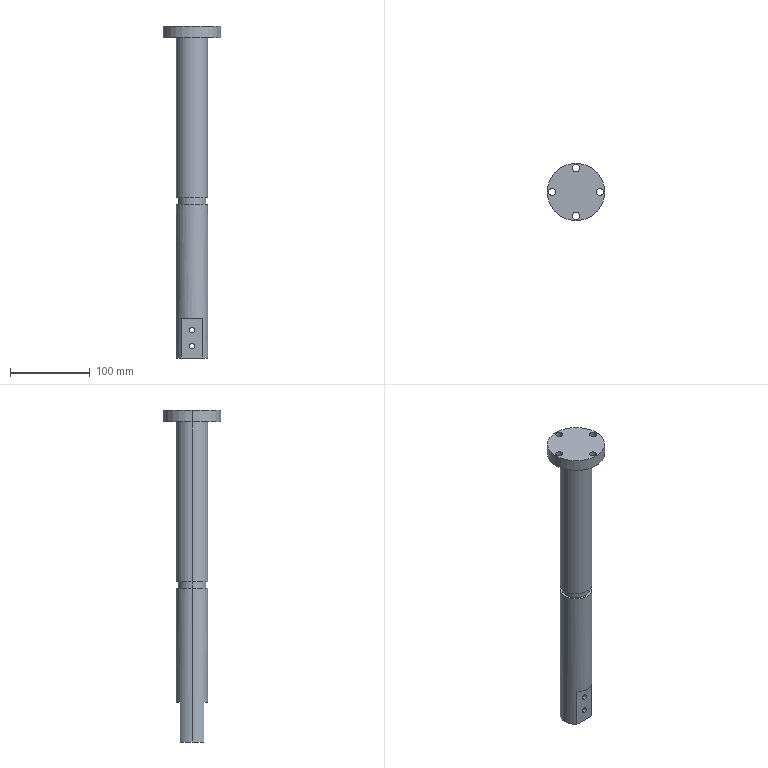Part | SolidWorks | features BaseBody 1 | 1 solid | 29 faces | box 72 x 72 x 416.14 mm | volume 547741 mm3 | cylinder 20 | plane 9 | commonest cylinder face diameters 9 x8 6.8 x4 40 x4 35 x2 72 x2
STEP:
#1=CARTESIAN_POINT('',(-20.,0.,-32.879));
#2=VERTEX_POINT('',#1);
#3=CARTESIAN_POINT('',(20.,0.,-32.879));
#4=VERTEX_POINT('',#3);
#5=CARTESIAN_POINT('',(0.,0.,-32.879));
#6=DIRECTION('',(0.,0.,-1.));
#7=DIRECTION('',(-1.,0.,0.));
#8=AXIS2_PLACEMENT_3D('',#5,#6,#7);
#9=CIRCLE('',#8,20.);
#10=EDGE_CURVE('',#2,#4,#9,.T.);
#11=ORIENTED_EDGE('',*,*,#10,.T.);
#12=CARTESIAN_POINT('',(20.,0.,-233.243));
#13=VERTEX_POINT('',#12);
#14=CARTESIAN_POINT('',(20.,0.,-32.879));
#15=DIRECTION('',(0.,0.,-1.));
#16=VECTOR('',#15,1000.);
#17=LINE('',#14,#16);
#18=EDGE_CURVE('',#4,#13,#17,.T.);
#19=ORIENTED_EDGE('',*,*,#18,.T.);
#20=CARTESIAN_POINT('',(-20.,0.,-233.243));
#21=VERTEX_POINT('',#20);
#22=CARTESIAN_POINT('',(0.,0.,-233.243));
#23=DIRECTION('',(0.,0.,1.));
#24=DIRECTION('',(-1.,0.,0.));
#25=AXIS2_PLACEMENT_3D('',#22,#23,#24);
#26=CIRCLE('',#25,20.);
#27=EDGE_CURVE('',#13,#21,#26,.T.);
#28=ORIENTED_EDGE('',*,*,#27,.T.);
#29=CARTESIAN_POINT('',(-20.,0.,-32.879));
#30=DIRECTION('',(0.,0.,-1.));
#31=VECTOR('',#30,1000.);
#32=LINE('',#29,#31);
#33=EDGE_CURVE('',#2,#21,#32,.T.);
#34=ORIENTED_EDGE('',*,*,#33,.F.);
#35=EDGE_LOOP('',(#11,#19,#28,#34));
#36=FACE_OUTER_BOUND('',#35,.T.);
#37=CARTESIAN_POINT('',(0.,0.,-32.879));
#38=DIRECTION('',(0.,0.,-1.));
#39=DIRECTION('',(-1.,0.,0.));
#40=AXIS2_PLACEMENT_3D('',#37,#38,#39);
#41=CYLINDRICAL_SURFACE('',#40,20.);
#42=ADVANCED_FACE('',(#36),#41,.T.);
#43=CARTESIAN_POINT('',(-17.5,0.,-233.243));
#44=VERTEX_POINT('',#43);
#45=CARTESIAN_POINT('',(17.5,0.,-233.243));
#46=VERTEX_POINT('',#45);
#47=CARTESIAN_POINT('',(0.,0.,-233.243));
#48=DIRECTION('',(0.,0.,-1.));
#49=DIRECTION('',(-1.,0.,0.));
#50=AXIS2_PLACEMENT_3D('',#47,#48,#49);
#51=CIRCLE('',#50,17.5);
#52=EDGE_CURVE('',#44,#46,#51,.T.);
#53=ORIENTED_EDGE('',*,*,#52,.T.);
#54=CARTESIAN_POINT('',(17.5,0.,-241.243));
#55=VERTEX_POINT('',#54);
#56=CARTESIAN_POINT('',(17.5,0.,-434.019));
#57=DIRECTION('',(0.,0.,-1.));
#58=VECTOR('',#57,1000.);
#59=LINE('',#56,#58);
#60=EDGE_CURVE('',#46,#55,#59,.T.);
#61=ORIENTED_EDGE('',*,*,#60,.T.);
#62=CARTESIAN_POINT('',(-17.5,0.,-241.243));
#63=VERTEX_POINT('',#62);
#64=CARTESIAN_POINT('',(0.,0.,-241.243));
#65=DIRECTION('',(0.,0.,1.));
#66=DIRECTION('',(-1.,0.,0.));
#67=AXIS2_PLACEMENT_3D('',#64,#65,#66);
#68=CIRCLE('',#67,17.5);
#69=EDGE_CURVE('',#55,#63,#68,.T.);
#70=ORIENTED_EDGE('',*,*,#69,.T.);
#71=CARTESIAN_POINT('',(-17.5,0.,-434.019));
#72=DIRECTION('',(0.,0.,-1.));
#73=VECTOR('',#72,1000.);
#74=LINE('',#71,#73);
#75=EDGE_CURVE('',#44,#63,#74,.T.);
#76=ORIENTED_EDGE('',*,*,#75,.F.);
#77=EDGE_LOOP('',(#53,#61,#70,#76));
#78=FACE_OUTER_BOUND('',#77,.T.);
#79=CARTESIAN_POINT('',(0.,0.,-434.019));
#80=DIRECTION('',(0.,0.,-1.));
#81=DIRECTION('',(-1.,0.,0.));
#82=AXIS2_PLACEMENT_3D('',#79,#80,#81);
#83=CYLINDRICAL_SURFACE('',#82,17.5);
#84=ADVANCED_FACE('',(#78),#83,.T.);
#85=CARTESIAN_POINT('',(-36.,0.,-17.879));
#86=VERTEX_POINT('',#85);
#87=CARTESIAN_POINT('',(36.,0.,-17.879));
#88=VERTEX_POINT('',#87);
#89=CARTESIAN_POINT('',(0.,0.,-17.879));
#90=DIRECTION('',(0.,0.,-1.));
#91=DIRECTION('',(-1.,0.,0.));
#92=AXIS2_PLACEMENT_3D('',#89,#90,#91);
#93=CIRCLE('',#92,36.);
#94=EDGE_CURVE('',#86,#88,#93,.T.);
#95=ORIENTED_EDGE('',*,*,#94,.T.);
#96=CARTESIAN_POINT('',(36.,0.,-32.879));
#97=VERTEX_POINT('',#96);
#98=CARTESIAN_POINT('',(36.,0.,-17.879));
#99=DIRECTION('',(0.,0.,-1.));
#100=VECTOR('',#99,1000.);
#101=LINE('',#98,#100);
#102=EDGE_CURVE('',#88,#97,#101,.T.);
#103=ORIENTED_EDGE('',*,*,#102,.T.);
#104=CARTESIAN_POINT('',(-36.,0.,-32.879));
#105=VERTEX_POINT('',#104);
#106=CARTESIAN_POINT('',(0.,0.,-32.879));
#107=DIRECTION('',(0.,0.,1.));
#108=DIRECTION('',(-1.,0.,0.));
#109=AXIS2_PLACEMENT_3D('',#106,#107,#108);
#110=CIRCLE('',#109,36.);
#111=EDGE_CURVE('',#97,#105,#110,.T.);
#112=ORIENTED_EDGE('',*,*,#111,.T.);
#113=CARTESIAN_POINT('',(-36.,0.,-17.879));
#114=DIRECTION('',(0.,0.,-1.));
#115=VECTOR('',#114,1000.);
#116=LINE('',#113,#115);
#117=EDGE_CURVE('',#86,#105,#116,.T.);
#118=ORIENTED_EDGE('',*,*,#117,.F.);
#119=EDGE_LOOP('',(#95,#103,#112,#118));
#120=FACE_OUTER_BOUND('',#119,.T.);
#121=CARTESIAN_POINT('',(0.,0.,-17.879));
#122=DIRECTION('',(0.,0.,-1.));
#123=DIRECTION('',(-1.,0.,0.));
#124=AXIS2_PLACEMENT_3D('',#121,#122,#123);
#125=CYLINDRICAL_SURFACE('',#124,36.);
#126=ADVANCED_FACE('',(#120),#125,.T.);
#127=CARTESIAN_POINT('',(4.5,30.,-32.879));
#128=VERTEX_POINT('',#127);
#129=CARTESIAN_POINT('',(-4.5,30.,-32.879));
#130=VERTEX_POINT('',#129);
#131=CARTESIAN_POINT('',(0.,30.,-32.879));
#132=DIRECTION('',(0.,0.,-1.));
#133=DIRECTION('',(1.,0.,0.));
#134=AXIS2_PLACEMENT_3D('',#131,#132,#133);
#135=CIRCLE('',#134,4.5);
#136=EDGE_CURVE('',#128,#130,#135,.T.);
#137=ORIENTED_EDGE('',*,*,#136,.T.);
#138=CARTESIAN_POINT('',(-4.5,30.,-17.879));
#139=VERTEX_POINT('',#138);
#140=CARTESIAN_POINT('',(-4.5,30.,-434.02));
#141=DIRECTION('',(0.,0.,1.));
#142=VECTOR('',#141,1000.);
#143=LINE('',#140,#142);
#144=EDGE_CURVE('',#130,#139,#143,.T.);
#145=ORIENTED_EDGE('',*,*,#144,.T.);
#146=CARTESIAN_POINT('',(4.5,30.,-17.879));
#147=VERTEX_POINT('',#146);
#148=CARTESIAN_POINT('',(0.,30.,-17.879));
#149=DIRECTION('',(0.,0.,-1.));
#150=DIRECTION('',(1.,0.,0.));
#151=AXIS2_PLACEMENT_3D('',#148,#149,#150);
#152=CIRCLE('',#151,4.5);
#153=EDGE_CURVE('',#147,#139,#152,.T.);
#154=ORIENTED_EDGE('',*,*,#153,.F.);
#155=CARTESIAN_POINT('',(4.5,30.,-434.02));
#156=DIRECTION('',(0.,0.,1.));
#157=VECTOR('',#156,1000.);
#158=LINE('',#155,#157);
#159=EDGE_CURVE('',#128,#147,#158,.T.);
#160=ORIENTED_EDGE('',*,*,#159,.F.);
#161=EDGE_LOOP('',(#137,#145,#154,#160));
#162=FACE_OUTER_BOUND('',#161,.T.);
#163=CARTESIAN_POINT('',(0.,30.,-434.02));
#164=DIRECTION('',(0.,0.,1.));
#165=DIRECTION('',(1.,0.,0.));
#166=AXIS2_PLACEMENT_3D('',#163,#164,#165);
#167=CYLINDRICAL_SURFACE('',#166,4.5);
#168=ADVANCED_FACE('',(#162),#167,.F.);
#169=CARTESIAN_POINT('',(-25.5,0.,-32.879));
#170=VERTEX_POINT('',#169);
#171=CARTESIAN_POINT('',(-34.5,0.,-32.879));
#172=VERTEX_POINT('',#171);
#173=CARTESIAN_POINT('',(-30.,0.,-32.879));
#174=DIRECTION('',(0.,0.,-1.));
#175=DIRECTION('',(1.,0.,0.));
#176=AXIS2_PLACEMENT_3D('',#173,#174,#175);
#177=CIRCLE('',#176,4.5);
#178=EDGE_CURVE('',#170,#172,#177,.T.);
#179=ORIENTED_EDGE('',*,*,#178,.T.);
#180=CARTESIAN_POINT('',(-34.5,0.,-17.879));
#181=VERTEX_POINT('',#180);
#182=CARTESIAN_POINT('',(-34.5,0.,-434.02));
#183=DIRECTION('',(0.,0.,1.));
#184=VECTOR('',#183,1000.);
#185=LINE('',#182,#184);
#186=EDGE_CURVE('',#172,#181,#185,.T.);
#187=ORIENTED_EDGE('',*,*,#186,.T.);
#188=CARTESIAN_POINT('',(-25.5,0.,-17.879));
#189=VERTEX_POINT('',#188);
#190=CARTESIAN_POINT('',(-30.,0.,-17.879));
#191=DIRECTION('',(0.,0.,-1.));
#192=DIRECTION('',(1.,0.,0.));
#193=AXIS2_PLACEMENT_3D('',#190,#191,#192);
#194=CIRCLE('',#193,4.5);
#195=EDGE_CURVE('',#189,#181,#194,.T.);
#196=ORIENTED_EDGE('',*,*,#195,.F.);
#197=CARTESIAN_POINT('',(-25.5,0.,-434.02));
#198=DIRECTION('',(0.,0.,1.));
#199=VECTOR('',#198,1000.);
#200=LINE('',#197,#199);
#201=EDGE_CURVE('',#170,#189,#200,.T.);
#202=ORIENTED_EDGE('',*,*,#201,.F.);
#203=EDGE_LOOP('',(#179,#187,#196,#202));
#204=FACE_OUTER_BOUND('',#203,.T.);
#205=CARTESIAN_POINT('',(-30.,0.,-434.02));
#206=DIRECTION('',(0.,0.,1.));
#207=DIRECTION('',(1.,0.,0.));
#208=AXIS2_PLACEMENT_3D('',#205,#206,#207);
#209=CYLINDRICAL_SURFACE('',#208,4.5);
#210=ADVANCED_FACE('',(#204),#209,.F.);
#211=CARTESIAN_POINT('',(4.5,-30.,-32.879));
#212=VERTEX_POINT('',#211);
#213=CARTESIAN_POINT('',(-4.5,-30.,-32.879));
#214=VERTEX_POINT('',#213);
#215=CARTESIAN_POINT('',(0.,-30.,-32.879));
#216=DIRECTION('',(0.,0.,-1.));
#217=DIRECTION('',(1.,0.,0.));
#218=AXIS2_PLACEMENT_3D('',#215,#216,#217);
#219=CIRCLE('',#218,4.5);
#220=EDGE_CURVE('',#212,#214,#219,.T.);
#221=ORIENTED_EDGE('',*,*,#220,.T.);
#222=CARTESIAN_POINT('',(-4.5,-30.,-17.879));
#223=VERTEX_POINT('',#222);
#224=CARTESIAN_POINT('',(-4.5,-30.,-434.02));
#225=DIRECTION('',(0.,0.,1.));
#226=VECTOR('',#225,1000.);
#227=LINE('',#224,#226);
#228=EDGE_CURVE('',#214,#223,#227,.T.);
#229=ORIENTED_EDGE('',*,*,#228,.T.);
#230=CARTESIAN_POINT('',(4.5,-30.,-17.879));
#231=VERTEX_POINT('',#230);
#232=CARTESIAN_POINT('',(0.,-30.,-17.879));
#233=DIRECTION('',(0.,0.,-1.));
#234=DIRECTION('',(1.,0.,0.));
#235=AXIS2_PLACEMENT_3D('',#232,#233,#234);
#236=CIRCLE('',#235,4.5);
#237=EDGE_CURVE('',#231,#223,#236,.T.);
#238=ORIENTED_EDGE('',*,*,#237,.F.);
#239=CARTESIAN_POINT('',(4.5,-30.,-434.02));
#240=DIRECTION('',(0.,0.,1.));
#241=VECTOR('',#240,1000.);
#242=LINE('',#239,#241);
#243=EDGE_CURVE('',#212,#231,#242,.T.);
#244=ORIENTED_EDGE('',*,*,#243,.F.);
#245=EDGE_LOOP('',(#221,#229,#238,#244));
#246=FACE_OUTER_BOUND('',#245,.T.);
#247=CARTESIAN_POINT('',(0.,-30.,-434.02));
#248=DIRECTION('',(0.,0.,1.));
#249=DIRECTION('',(1.,0.,0.));
#250=AXIS2_PLACEMENT_3D('',#247,#248,#249);
#251=CYLINDRICAL_SURFACE('',#250,4.5);
#252=ADVANCED_FACE('',(#246),#251,.F.);
#253=CARTESIAN_POINT('',(34.5,0.,-32.879));
#254=VERTEX_POINT('',#253);
#255=CARTESIAN_POINT('',(25.5,0.,-32.879));
#256=VERTEX_POINT('',#255);
#257=CARTESIAN_POINT('',(30.,0.,-32.879));
#258=DIRECTION('',(0.,0.,-1.));
#259=DIRECTION('',(1.,0.,0.));
#260=AXIS2_PLACEMENT_3D('',#257,#258,#259);
#261=CIRCLE('',#260,4.5);
#262=EDGE_CURVE('',#254,#256,#261,.T.);
#263=ORIENTED_EDGE('',*,*,#262,.T.);
#264=CARTESIAN_POINT('',(25.5,0.,-17.879));
#265=VERTEX_POINT('',#264);
#266=CARTESIAN_POINT('',(25.5,0.,-434.02));
#267=DIRECTION('',(0.,0.,1.));
#268=VECTOR('',#267,1000.);
#269=LINE('',#266,#268);
#270=EDGE_CURVE('',#256,#265,#269,.T.);
#271=ORIENTED_EDGE('',*,*,#270,.T.);
#272=CARTESIAN_POINT('',(34.5,0.,-17.879));
#273=VERTEX_POINT('',#272);
#274=CARTESIAN_POINT('',(30.,0.,-17.879));
#275=DIRECTION('',(0.,0.,-1.));
#276=DIRECTION('',(1.,0.,0.));
#277=AXIS2_PLACEMENT_3D('',#274,#275,#276);
#278=CIRCLE('',#277,4.5);
#279=EDGE_CURVE('',#273,#265,#278,.T.);
#280=ORIENTED_EDGE('',*,*,#279,.F.);
#281=CARTESIAN_POINT('',(34.5,0.,-434.02));
#282=DIRECTION('',(0.,0.,1.));
#283=VECTOR('',#282,1000.);
#284=LINE('',#281,#283);
#285=EDGE_CURVE('',#254,#273,#284,.T.);
#286=ORIENTED_EDGE('',*,*,#285,.F.);
#287=EDGE_LOOP('',(#263,#271,#280,#286));
#288=FACE_OUTER_BOUND('',#287,.T.);
#289=CARTESIAN_POINT('',(30.,0.,-434.02));
#290=DIRECTION('',(0.,0.,1.));
#291=DIRECTION('',(1.,0.,0.));
#292=AXIS2_PLACEMENT_3D('',#289,#290,#291);
#293=CYLINDRICAL_SURFACE('',#292,4.5);
#294=ADVANCED_FACE('',(#288),#293,.F.);
#295=CARTESIAN_POINT('',(20.,0.,-241.243));
#296=VERTEX_POINT('',#295);
#297=CARTESIAN_POINT('',(-20.,0.,-241.243));
#298=VERTEX_POINT('',#297);
#299=CARTESIAN_POINT('',(0.,0.,-241.243));
#300=DIRECTION('',(0.,0.,1.));
#301=DIRECTION('',(-1.,0.,0.));
#302=AXIS2_PLACEMENT_3D('',#299,#300,#301);
#303=CIRCLE('',#302,20.);
#304=EDGE_CURVE('',#296,#298,#303,.T.);
#305=ORIENTED_EDGE('',*,*,#304,.F.);
#306=CARTESIAN_POINT('',(20.,0.,-434.019));
#307=VERTEX_POINT('',#306);
#308=CARTESIAN_POINT('',(20.,0.,-32.879));
#309=DIRECTION('',(0.,0.,-1.));
#310=VECTOR('',#309,1000.);
#311=LINE('',#308,#310);
#312=EDGE_CURVE('',#296,#307,#311,.T.);
#313=ORIENTED_EDGE('',*,*,#312,.T.);
#314=CARTESIAN_POINT('',(13.229,15.,-434.019));
#315=VERTEX_POINT('',#314);
#316=CARTESIAN_POINT('',(0.,0.,-434.019));
#317=DIRECTION('',(0.,0.,1.));
#318=DIRECTION('',(-1.,0.,0.));
#319=AXIS2_PLACEMENT_3D('',#316,#317,#318);
#320=CIRCLE('',#319,20.);
#321=EDGE_CURVE('',#307,#315,#320,.T.);
#322=ORIENTED_EDGE('',*,*,#321,.T.);
#323=CARTESIAN_POINT('',(13.229,15.,-384.019));
#324=VERTEX_POINT('',#323);
#325=CARTESIAN_POINT('',(13.229,15.,-32.879));
#326=DIRECTION('',(0.,0.,1.));
#327=VECTOR('',#326,1000.);
#328=LINE('',#325,#327);
#329=EDGE_CURVE('',#315,#324,#328,.T.);
#330=ORIENTED_EDGE('',*,*,#329,.T.);
#331=CARTESIAN_POINT('',(-13.229,15.,-384.019));
#332=VERTEX_POINT('',#331);
#333=CARTESIAN_POINT('',(0.,0.,-384.019));
#334=DIRECTION('',(0.,0.,1.));
#335=DIRECTION('',(-1.,0.,0.));
#336=AXIS2_PLACEMENT_3D('',#333,#334,#335);
#337=CIRCLE('',#336,20.);
#338=EDGE_CURVE('',#324,#332,#337,.T.);
#339=ORIENTED_EDGE('',*,*,#338,.T.);
#340=CARTESIAN_POINT('',(-13.229,15.,-434.019));
#341=VERTEX_POINT('',#340);
#342=CARTESIAN_POINT('',(-13.229,15.,-32.879));
#343=DIRECTION('',(0.,0.,-1.));
#344=VECTOR('',#343,1000.);
#345=LINE('',#342,#344);
#346=EDGE_CURVE('',#332,#341,#345,.T.);
#347=ORIENTED_EDGE('',*,*,#346,.T.);
#348=CARTESIAN_POINT('',(-20.,0.,-434.019));
#349=VERTEX_POINT('',#348);
#350=CARTESIAN_POINT('',(0.,0.,-434.019));
#351=DIRECTION('',(0.,0.,1.));
#352=DIRECTION('',(-1.,0.,0.));
#353=AXIS2_PLACEMENT_3D('',#350,#351,#352);
#354=CIRCLE('',#353,20.);
#355=EDGE_CURVE('',#341,#349,#354,.T.);
#356=ORIENTED_EDGE('',*,*,#355,.T.);
#357=CARTESIAN_POINT('',(-20.,0.,-32.879));
#358=DIRECTION('',(0.,0.,-1.));
#359=VECTOR('',#358,1000.);
#360=LINE('',#357,#359);
#361=EDGE_CURVE('',#298,#349,#360,.T.);
#362=ORIENTED_EDGE('',*,*,#361,.F.);
#363=EDGE_LOOP('',(#305,#313,#322,#330,#339,#347,#356,#362));
#364=FACE_OUTER_BOUND('',#363,.T.);
#365=CARTESIAN_POINT('',(0.,0.,-32.879));
#366=DIRECTION('',(0.,0.,-1.));
#367=DIRECTION('',(-1.,0.,0.));
#368=AXIS2_PLACEMENT_3D('',#365,#366,#367);
#369=CYLINDRICAL_SURFACE('',#368,20.);
#370=ADVANCED_FACE('',(#364),#369,.T.);
#371=CARTESIAN_POINT('',(0.,-15.,-422.419));
#372=VERTEX_POINT('',#371);
#373=CARTESIAN_POINT('',(0.,-15.,-415.619));
#374=VERTEX_POINT('',#373);
#375=CARTESIAN_POINT('',(0.,-15.,-419.019));
#376=DIRECTION('',(0.,1.,0.));
#377=DIRECTION('',(0.,0.,1.));
#378=AXIS2_PLACEMENT_3D('',#375,#376,#377);
#379=CIRCLE('',#378,3.4);
#380=EDGE_CURVE('',#372,#374,#379,.T.);
#381=ORIENTED_EDGE('',*,*,#380,.F.);
#382=CARTESIAN_POINT('',(0.,15.,-422.419));
#383=VERTEX_POINT('',#382);
#384=CARTESIAN_POINT('',(0.,15.,-422.419));
#385=DIRECTION('',(0.,1.,0.));
#386=VECTOR('',#385,1000.);
#387=LINE('',#384,#386);
#388=EDGE_CURVE('',#372,#383,#387,.T.);
#389=ORIENTED_EDGE('',*,*,#388,.T.);
#390=CARTESIAN_POINT('',(0.,15.,-415.619));
#391=VERTEX_POINT('',#390);
#392=CARTESIAN_POINT('',(0.,15.,-419.019));
#393=DIRECTION('',(0.,1.,0.));
#394=DIRECTION('',(0.,0.,1.));
#395=AXIS2_PLACEMENT_3D('',#392,#393,#394);
#396=CIRCLE('',#395,3.4);
#397=EDGE_CURVE('',#383,#391,#396,.T.);
#398=ORIENTED_EDGE('',*,*,#397,.T.);
#399=CARTESIAN_POINT('',(0.,15.,-415.619));
#400=DIRECTION('',(0.,1.,0.));
#401=VECTOR('',#400,1000.);
#402=LINE('',#399,#401);
#403=EDGE_CURVE('',#374,#391,#402,.T.);
#404=ORIENTED_EDGE('',*,*,#403,.F.);
#405=EDGE_LOOP('',(#381,#389,#398,#404));
#406=FACE_OUTER_BOUND('',#405,.T.);
#407=CARTESIAN_POINT('',(0.,15.,-419.019));
#408=DIRECTION('',(0.,1.,0.));
#409=DIRECTION('',(0.,0.,1.));
#410=AXIS2_PLACEMENT_3D('',#407,#408,#409);
#411=CYLINDRICAL_SURFACE('',#410,3.4);
#412=ADVANCED_FACE('',(#406),#411,.F.);
#413=CARTESIAN_POINT('',(0.,-15.,-402.419));
#414=VERTEX_POINT('',#413);
#415=CARTESIAN_POINT('',(0.,-15.,-395.619));
#416=VERTEX_POINT('',#415);
#417=CARTESIAN_POINT('',(0.,-15.,-399.019));
#418=DIRECTION('',(0.,1.,0.));
#419=DIRECTION('',(0.,0.,1.));
#420=AXIS2_PLACEMENT_3D('',#417,#418,#419);
#421=CIRCLE('',#420,3.4);
#422=EDGE_CURVE('',#414,#416,#421,.T.);
#423=ORIENTED_EDGE('',*,*,#422,.F.);
#424=CARTESIAN_POINT('',(0.,15.,-402.419));
#425=VERTEX_POINT('',#424);
#426=CARTESIAN_POINT('',(0.,15.,-402.419));
#427=DIRECTION('',(0.,1.,0.));
#428=VECTOR('',#427,1000.);
#429=LINE('',#426,#428);
#430=EDGE_CURVE('',#414,#425,#429,.T.);
#431=ORIENTED_EDGE('',*,*,#430,.T.);
#432=CARTESIAN_POINT('',(0.,15.,-395.619));
#433=VERTEX_POINT('',#432);
#434=CARTESIAN_POINT('',(0.,15.,-399.019));
#435=DIRECTION('',(0.,1.,0.));
#436=DIRECTION('',(0.,0.,1.));
#437=AXIS2_PLACEMENT_3D('',#434,#435,#436);
#438=CIRCLE('',#437,3.4);
#439=EDGE_CURVE('',#425,#433,#438,.T.);
#440=ORIENTED_EDGE('',*,*,#439,.T.);
#441=CARTESIAN_POINT('',(0.,15.,-395.619));
#442=DIRECTION('',(0.,1.,0.));
#443=VECTOR('',#442,1000.);
#444=LINE('',#441,#443);
#445=EDGE_CURVE('',#416,#433,#444,.T.);
#446=ORIENTED_EDGE('',*,*,#445,.F.);
#447=EDGE_LOOP('',(#423,#431,#440,#446));
#448=FACE_OUTER_BOUND('',#447,.T.);
#449=CARTESIAN_POINT('',(0.,15.,-399.019));
#450=DIRECTION('',(0.,1.,0.));
#451=DIRECTION('',(0.,0.,1.));
#452=AXIS2_PLACEMENT_3D('',#449,#450,#451);
#453=CYLINDRICAL_SURFACE('',#452,3.4);
#454=ADVANCED_FACE('',(#448),#453,.F.);
#455=ORIENTED_EDGE('',*,*,#18,.F.);
#456=CARTESIAN_POINT('',(0.,0.,-32.879));
#457=DIRECTION('',(0.,0.,-1.));
#458=DIRECTION('',(-1.,0.,0.));
#459=AXIS2_PLACEMENT_3D('',#456,#457,#458);
#460=CIRCLE('',#459,20.);
#461=EDGE_CURVE('',#4,#2,#460,.T.);
#462=ORIENTED_EDGE('',*,*,#461,.T.);
#463=ORIENTED_EDGE('',*,*,#33,.T.);
#464=CARTESIAN_POINT('',(0.,0.,-233.243));
#465=DIRECTION('',(0.,0.,1.));
#466=DIRECTION('',(-1.,0.,0.));
#467=AXIS2_PLACEMENT_3D('',#464,#465,#466);
#468=CIRCLE('',#467,20.);
#469=EDGE_CURVE('',#21,#13,#468,.T.);
#470=ORIENTED_EDGE('',*,*,#469,.T.);
#471=EDGE_LOOP('',(#455,#462,#463,#470));
#472=FACE_OUTER_BOUND('',#471,.T.);
#473=CARTESIAN_POINT('',(0.,0.,-32.879));
#474=DIRECTION('',(0.,0.,-1.));
#475=DIRECTION('',(-1.,0.,0.));
#476=AXIS2_PLACEMENT_3D('',#473,#474,#475);
#477=CYLINDRICAL_SURFACE('',#476,20.);
#478=ADVANCED_FACE('',(#472),#477,.T.);
#479=ORIENTED_EDGE('',*,*,#469,.F.);
#480=ORIENTED_EDGE('',*,*,#27,.F.);
#481=EDGE_LOOP('',(#479,#480));
#482=FACE_OUTER_BOUND('',#481,.T.);
#483=ORIENTED_EDGE('',*,*,#52,.F.);
#484=CARTESIAN_POINT('',(0.,0.,-233.243));
#485=DIRECTION('',(0.,0.,-1.));
#486=DIRECTION('',(-1.,0.,0.));
#487=AXIS2_PLACEMENT_3D('',#484,#485,#486);
#488=CIRCLE('',#487,17.5);
#489=EDGE_CURVE('',#46,#44,#488,.T.);
#490=ORIENTED_EDGE('',*,*,#489,.F.);
#491=EDGE_LOOP('',(#483,#490));
#492=FACE_BOUND('',#491,.T.);
#493=CARTESIAN_POINT('',(0.,-20.,-233.243));
#494=DIRECTION('',(0.,0.,1.));
#495=DIRECTION('',(1.,0.,0.));
#496=AXIS2_PLACEMENT_3D('',#493,#494,#495);
#497=PLANE('',#496);
#498=ADVANCED_FACE('',(#482,#492),#497,.F.);
#499=ORIENTED_EDGE('',*,*,#10,.F.);
#500=ORIENTED_EDGE('',*,*,#461,.F.);
#501=EDGE_LOOP('',(#499,#500));
#502=FACE_BOUND('',#501,.T.);
#503=CARTESIAN_POINT('',(0.,0.,-32.879));
#504=DIRECTION('',(0.,0.,1.));
#505=DIRECTION('',(-1.,0.,0.));
#506=AXIS2_PLACEMENT_3D('',#503,#504,#505);
#507=CIRCLE('',#506,36.);
#508=EDGE_CURVE('',#105,#97,#507,.T.);
#509=ORIENTED_EDGE('',*,*,#508,.F.);
#510=ORIENTED_EDGE('',*,*,#111,.F.);
#511=EDGE_LOOP('',(#509,#510));
#512=FACE_OUTER_BOUND('',#511,.T.);
#513=ORIENTED_EDGE('',*,*,#136,.F.);
#514=CARTESIAN_POINT('',(0.,30.,-32.879));
#515=DIRECTION('',(0.,0.,-1.));
#516=DIRECTION('',(1.,0.,0.));
#517=AXIS2_PLACEMENT_3D('',#514,#515,#516);
#518=CIRCLE('',#517,4.5);
#519=EDGE_CURVE('',#130,#128,#518,.T.);
#520=ORIENTED_EDGE('',*,*,#519,.F.);
#521=EDGE_LOOP('',(#513,#520));
#522=FACE_BOUND('',#521,.T.);
#523=ORIENTED_EDGE('',*,*,#178,.F.);
#524=CARTESIAN_POINT('',(-30.,0.,-32.879));
#525=DIRECTION('',(0.,0.,-1.));
#526=DIRECTION('',(1.,0.,0.));
#527=AXIS2_PLACEMENT_3D('',#524,#525,#526);
#528=CIRCLE('',#527,4.5);
#529=EDGE_CURVE('',#172,#170,#528,.T.);
#530=ORIENTED_EDGE('',*,*,#529,.F.);
#531=EDGE_LOOP('',(#523,#530));
#532=FACE_BOUND('',#531,.T.);
#533=ORIENTED_EDGE('',*,*,#220,.F.);
#534=CARTESIAN_POINT('',(0.,-30.,-32.879));
#535=DIRECTION('',(0.,0.,-1.));
#536=DIRECTION('',(1.,0.,0.));
#537=AXIS2_PLACEMENT_3D('',#534,#535,#536);
#538=CIRCLE('',#537,4.5);
#539=EDGE_CURVE('',#214,#212,#538,.T.);
#540=ORIENTED_EDGE('',*,*,#539,.F.);
#541=EDGE_LOOP('',(#533,#540));
#542=FACE_BOUND('',#541,.T.);
#543=ORIENTED_EDGE('',*,*,#262,.F.);
#544=CARTESIAN_POINT('',(30.,0.,-32.879));
#545=DIRECTION('',(0.,0.,-1.));
#546=DIRECTION('',(1.,0.,0.));
#547=AXIS2_PLACEMENT_3D('',#544,#545,#546);
#548=CIRCLE('',#547,4.5);
#549=EDGE_CURVE('',#256,#254,#548,.T.);
#550=ORIENTED_EDGE('',*,*,#549,.F.);
#551=EDGE_LOOP('',(#543,#550));
#552=FACE_BOUND('',#551,.T.);
#553=CARTESIAN_POINT('',(0.,0.,-32.879));
#554=DIRECTION('',(0.,0.,1.));
#555=DIRECTION('',(1.,0.,0.));
#556=AXIS2_PLACEMENT_3D('',#553,#554,#555);
#557=PLANE('',#556);
#558=ADVANCED_FACE('',(#502,#512,#522,#532,#542,#552),#557,.F.);
#559=ORIENTED_EDGE('',*,*,#60,.F.);
#560=ORIENTED_EDGE('',*,*,#489,.T.);
#561=ORIENTED_EDGE('',*,*,#75,.T.);
#562=CARTESIAN_POINT('',(0.,0.,-241.243));
#563=DIRECTION('',(0.,0.,1.));
#564=DIRECTION('',(-1.,0.,0.));
#565=AXIS2_PLACEMENT_3D('',#562,#563,#564);
#566=CIRCLE('',#565,17.5);
#567=EDGE_CURVE('',#63,#55,#566,.T.);
#568=ORIENTED_EDGE('',*,*,#567,.T.);
#569=EDGE_LOOP('',(#559,#560,#561,#568));
#570=FACE_OUTER_BOUND('',#569,.T.);
#571=CARTESIAN_POINT('',(0.,0.,-434.019));
#572=DIRECTION('',(0.,0.,-1.));
#573=DIRECTION('',(-1.,0.,0.));
#574=AXIS2_PLACEMENT_3D('',#571,#572,#573);
#575=CYLINDRICAL_SURFACE('',#574,17.5);
#576=ADVANCED_FACE('',(#570),#575,.T.);
#577=ORIENTED_EDGE('',*,*,#102,.F.);
#578=CARTESIAN_POINT('',(0.,0.,-17.879));
#579=DIRECTION('',(0.,0.,-1.));
#580=DIRECTION('',(-1.,0.,0.));
#581=AXIS2_PLACEMENT_3D('',#578,#579,#580);
#582=CIRCLE('',#581,36.);
#583=EDGE_CURVE('',#88,#86,#582,.T.);
#584=ORIENTED_EDGE('',*,*,#583,.T.);
#585=ORIENTED_EDGE('',*,*,#117,.T.);
#586=ORIENTED_EDGE('',*,*,#508,.T.);
#587=EDGE_LOOP('',(#577,#584,#585,#586));
#588=FACE_OUTER_BOUND('',#587,.T.);
#589=CARTESIAN_POINT('',(0.,0.,-17.879));
#590=DIRECTION('',(0.,0.,-1.));
#591=DIRECTION('',(-1.,0.,0.));
#592=AXIS2_PLACEMENT_3D('',#589,#590,#591);
#593=CYLINDRICAL_SURFACE('',#592,36.);
#594=ADVANCED_FACE('',(#588),#593,.T.);
#595=ORIENTED_EDGE('',*,*,#144,.F.);
#596=ORIENTED_EDGE('',*,*,#519,.T.);
#597=ORIENTED_EDGE('',*,*,#159,.T.);
#598=CARTESIAN_POINT('',(0.,30.,-17.879));
#599=DIRECTION('',(0.,0.,-1.));
#600=DIRECTION('',(1.,0.,0.));
#601=AXIS2_PLACEMENT_3D('',#598,#599,#600);
#602=CIRCLE('',#601,4.5);
#603=EDGE_CURVE('',#139,#147,#602,.T.);
#604=ORIENTED_EDGE('',*,*,#603,.F.);
#605=EDGE_LOOP('',(#595,#596,#597,#604));
#606=FACE_OUTER_BOUND('',#605,.T.);
#607=CARTESIAN_POINT('',(0.,30.,-434.02));
#608=DIRECTION('',(0.,0.,1.));
#609=DIRECTION('',(1.,0.,0.));
#610=AXIS2_PLACEMENT_3D('',#607,#608,#609);
#611=CYLINDRICAL_SURFACE('',#610,4.5);
#612=ADVANCED_FACE('',(#606),#611,.F.);
#613=ORIENTED_EDGE('',*,*,#186,.F.);
#614=ORIENTED_EDGE('',*,*,#529,.T.);
#615=ORIENTED_EDGE('',*,*,#201,.T.);
#616=CARTESIAN_POINT('',(-30.,0.,-17.879));
#617=DIRECTION('',(0.,0.,-1.));
#618=DIRECTION('',(1.,0.,0.));
#619=AXIS2_PLACEMENT_3D('',#616,#617,#618);
#620=CIRCLE('',#619,4.5);
#621=EDGE_CURVE('',#181,#189,#620,.T.);
#622=ORIENTED_EDGE('',*,*,#621,.F.);
#623=EDGE_LOOP('',(#613,#614,#615,#622));
#624=FACE_OUTER_BOUND('',#623,.T.);
#625=CARTESIAN_POINT('',(-30.,0.,-434.02));
#626=DIRECTION('',(0.,0.,1.));
#627=DIRECTION('',(1.,0.,0.));
#628=AXIS2_PLACEMENT_3D('',#625,#626,#627);
#629=CYLINDRICAL_SURFACE('',#628,4.5);
#630=ADVANCED_FACE('',(#624),#629,.F.);
#631=ORIENTED_EDGE('',*,*,#228,.F.);
#632=ORIENTED_EDGE('',*,*,#539,.T.);
#633=ORIENTED_EDGE('',*,*,#243,.T.);
#634=CARTESIAN_POINT('',(0.,-30.,-17.879));
#635=DIRECTION('',(0.,0.,-1.));
#636=DIRECTION('',(1.,0.,0.));
#637=AXIS2_PLACEMENT_3D('',#634,#635,#636);
#638=CIRCLE('',#637,4.5);
#639=EDGE_CURVE('',#223,#231,#638,.T.);
#640=ORIENTED_EDGE('',*,*,#639,.F.);
#641=EDGE_LOOP('',(#631,#632,#633,#640));
#642=FACE_OUTER_BOUND('',#641,.T.);
#643=CARTESIAN_POINT('',(0.,-30.,-434.02));
#644=DIRECTION('',(0.,0.,1.));
#645=DIRECTION('',(1.,0.,0.));
#646=AXIS2_PLACEMENT_3D('',#643,#644,#645);
#647=CYLINDRICAL_SURFACE('',#646,4.5);
#648=ADVANCED_FACE('',(#642),#647,.F.);
#649=ORIENTED_EDGE('',*,*,#270,.F.);
#650=ORIENTED_EDGE('',*,*,#549,.T.);
#651=ORIENTED_EDGE('',*,*,#285,.T.);
#652=CARTESIAN_POINT('',(30.,0.,-17.879));
#653=DIRECTION('',(0.,0.,-1.));
#654=DIRECTION('',(1.,0.,0.));
#655=AXIS2_PLACEMENT_3D('',#652,#653,#654);
#656=CIRCLE('',#655,4.5);
#657=EDGE_CURVE('',#265,#273,#656,.T.);
#658=ORIENTED_EDGE('',*,*,#657,.F.);
#659=EDGE_LOOP('',(#649,#650,#651,#658));
#660=FACE_OUTER_BOUND('',#659,.T.);
#661=CARTESIAN_POINT('',(30.,0.,-434.02));
#662=DIRECTION('',(0.,0.,1.));
#663=DIRECTION('',(1.,0.,0.));
#664=AXIS2_PLACEMENT_3D('',#661,#662,#663);
#665=CYLINDRICAL_SURFACE('',#664,4.5);
#666=ADVANCED_FACE('',(#660),#665,.F.);
#667=CARTESIAN_POINT('',(0.,0.,-241.243));
#668=DIRECTION('',(0.,0.,1.));
#669=DIRECTION('',(-1.,0.,0.));
#670=AXIS2_PLACEMENT_3D('',#667,#668,#669);
#671=CIRCLE('',#670,20.);
#672=EDGE_CURVE('',#298,#296,#671,.T.);
#673=ORIENTED_EDGE('',*,*,#672,.T.);
#674=ORIENTED_EDGE('',*,*,#304,.T.);
#675=EDGE_LOOP('',(#673,#674));
#676=FACE_OUTER_BOUND('',#675,.T.);
#677=ORIENTED_EDGE('',*,*,#567,.F.);
#678=ORIENTED_EDGE('',*,*,#69,.F.);
#679=EDGE_LOOP('',(#677,#678));
#680=FACE_BOUND('',#679,.T.);
#681=CARTESIAN_POINT('',(0.,-20.,-241.243));
#682=DIRECTION('',(0.,0.,1.));
#683=DIRECTION('',(1.,0.,0.));
#684=AXIS2_PLACEMENT_3D('',#681,#682,#683);
#685=PLANE('',#684);
#686=ADVANCED_FACE('',(#676,#680),#685,.T.);
#687=ORIENTED_EDGE('',*,*,#94,.F.);
#688=ORIENTED_EDGE('',*,*,#583,.F.);
#689=EDGE_LOOP('',(#687,#688));
#690=FACE_OUTER_BOUND('',#689,.T.);
#691=ORIENTED_EDGE('',*,*,#153,.T.);
#692=ORIENTED_EDGE('',*,*,#603,.T.);
#693=EDGE_LOOP('',(#691,#692));
#694=FACE_BOUND('',#693,.T.);
#695=ORIENTED_EDGE('',*,*,#195,.T.);
#696=ORIENTED_EDGE('',*,*,#621,.T.);
#697=EDGE_LOOP('',(#695,#696));
#698=FACE_BOUND('',#697,.T.);
#699=ORIENTED_EDGE('',*,*,#237,.T.);
#700=ORIENTED_EDGE('',*,*,#639,.T.);
#701=EDGE_LOOP('',(#699,#700));
#702=FACE_BOUND('',#701,.T.);
#703=ORIENTED_EDGE('',*,*,#279,.T.);
#704=ORIENTED_EDGE('',*,*,#657,.T.);
#705=EDGE_LOOP('',(#703,#704));
#706=FACE_BOUND('',#705,.T.);
#707=CARTESIAN_POINT('',(0.,0.,-17.879));
#708=DIRECTION('',(0.,0.,1.));
#709=DIRECTION('',(1.,0.,0.));
#710=AXIS2_PLACEMENT_3D('',#707,#708,#709);
#711=PLANE('',#710);
#712=ADVANCED_FACE('',(#690,#694,#698,#702,#706),#711,.T.);
#713=ORIENTED_EDGE('',*,*,#312,.F.);
#714=ORIENTED_EDGE('',*,*,#672,.F.);
#715=ORIENTED_EDGE('',*,*,#361,.T.);
#716=CARTESIAN_POINT('',(-13.229,-15.,-434.019));
#717=VERTEX_POINT('',#716);
#718=CARTESIAN_POINT('',(0.,0.,-434.019));
#719=DIRECTION('',(0.,0.,1.));
#720=DIRECTION('',(-1.,0.,0.));
#721=AXIS2_PLACEMENT_3D('',#718,#719,#720);
#722=CIRCLE('',#721,20.);
#723=EDGE_CURVE('',#349,#717,#722,.T.);
#724=ORIENTED_EDGE('',*,*,#723,.T.);
#725=CARTESIAN_POINT('',(-13.229,-15.,-384.019));
#726=VERTEX_POINT('',#725);
#727=CARTESIAN_POINT('',(-13.229,-15.,-32.879));
#728=DIRECTION('',(0.,0.,1.));
#729=VECTOR('',#728,1000.);
#730=LINE('',#727,#729);
#731=EDGE_CURVE('',#717,#726,#730,.T.);
#732=ORIENTED_EDGE('',*,*,#731,.T.);
#733=CARTESIAN_POINT('',(13.229,-15.,-384.019));
#734=VERTEX_POINT('',#733);
#735=CARTESIAN_POINT('',(0.,0.,-384.019));
#736=DIRECTION('',(0.,0.,1.));
#737=DIRECTION('',(-1.,0.,0.));
#738=AXIS2_PLACEMENT_3D('',#735,#736,#737);
#739=CIRCLE('',#738,20.);
#740=EDGE_CURVE('',#726,#734,#739,.T.);
#741=ORIENTED_EDGE('',*,*,#740,.T.);
#742=CARTESIAN_POINT('',(13.229,-15.,-434.019));
#743=VERTEX_POINT('',#742);
#744=CARTESIAN_POINT('',(13.229,-15.,-32.879));
#745=DIRECTION('',(0.,0.,-1.));
#746=VECTOR('',#745,1000.);
#747=LINE('',#744,#746);
#748=EDGE_CURVE('',#734,#743,#747,.T.);
#749=ORIENTED_EDGE('',*,*,#748,.T.);
#750=CARTESIAN_POINT('',(0.,0.,-434.019));
#751=DIRECTION('',(0.,0.,1.));
#752=DIRECTION('',(-1.,0.,0.));
#753=AXIS2_PLACEMENT_3D('',#750,#751,#752);
#754=CIRCLE('',#753,20.);
#755=EDGE_CURVE('',#743,#307,#754,.T.);
#756=ORIENTED_EDGE('',*,*,#755,.T.);
#757=EDGE_LOOP('',(#713,#714,#715,#724,#732,#741,#749,#756));
#758=FACE_OUTER_BOUND('',#757,.T.);
#759=CARTESIAN_POINT('',(0.,0.,-32.879));
#760=DIRECTION('',(0.,0.,-1.));
#761=DIRECTION('',(-1.,0.,0.));
#762=AXIS2_PLACEMENT_3D('',#759,#760,#761);
#763=CYLINDRICAL_SURFACE('',#762,20.);
#764=ADVANCED_FACE('',(#758),#763,.T.);
#765=ORIENTED_EDGE('',*,*,#740,.F.);
#766=CARTESIAN_POINT('',(-50.,-15.,-384.019));
#767=DIRECTION('',(1.,0.,0.));
#768=VECTOR('',#767,1000.);
#769=LINE('',#766,#768);
#770=EDGE_CURVE('',#726,#734,#769,.T.);
#771=ORIENTED_EDGE('',*,*,#770,.T.);
#772=EDGE_LOOP('',(#765,#771));
#773=FACE_OUTER_BOUND('',#772,.T.);
#774=CARTESIAN_POINT('',(-50.,-29.781,-384.019));
#775=DIRECTION('',(0.,0.,-1.));
#776=DIRECTION('',(-1.,0.,0.));
#777=AXIS2_PLACEMENT_3D('',#774,#775,#776);
#778=PLANE('',#777);
#779=ADVANCED_FACE('',(#773),#778,.T.);
#780=ORIENTED_EDGE('',*,*,#748,.F.);
#781=ORIENTED_EDGE('',*,*,#770,.F.);
#782=ORIENTED_EDGE('',*,*,#731,.F.);
#783=CARTESIAN_POINT('',(-50.,-15.,-434.019));
#784=DIRECTION('',(1.,0.,0.));
#785=VECTOR('',#784,1000.);
#786=LINE('',#783,#785);
#787=EDGE_CURVE('',#717,#743,#786,.T.);
#788=ORIENTED_EDGE('',*,*,#787,.T.);
#789=EDGE_LOOP('',(#780,#781,#782,#788));
#790=FACE_OUTER_BOUND('',#789,.T.);
#791=CARTESIAN_POINT('',(0.,-15.,-419.019));
#792=DIRECTION('',(0.,1.,0.));
#793=DIRECTION('',(0.,0.,1.));
#794=AXIS2_PLACEMENT_3D('',#791,#792,#793);
#795=CIRCLE('',#794,3.4);
#796=EDGE_CURVE('',#374,#372,#795,.T.);
#797=ORIENTED_EDGE('',*,*,#796,.T.);
#798=ORIENTED_EDGE('',*,*,#380,.T.);
#799=EDGE_LOOP('',(#797,#798));
#800=FACE_BOUND('',#799,.T.);
#801=CARTESIAN_POINT('',(0.,-15.,-399.019));
#802=DIRECTION('',(0.,1.,0.));
#803=DIRECTION('',(0.,0.,1.));
#804=AXIS2_PLACEMENT_3D('',#801,#802,#803);
#805=CIRCLE('',#804,3.4);
#806=EDGE_CURVE('',#416,#414,#805,.T.);
#807=ORIENTED_EDGE('',*,*,#806,.T.);
#808=ORIENTED_EDGE('',*,*,#422,.T.);
#809=EDGE_LOOP('',(#807,#808));
#810=FACE_BOUND('',#809,.T.);
#811=CARTESIAN_POINT('',(-50.,-15.,-384.019));
#812=DIRECTION('',(0.,-1.,0.));
#813=DIRECTION('',(0.,0.,-1.));
#814=AXIS2_PLACEMENT_3D('',#811,#812,#813);
#815=PLANE('',#814);
#816=ADVANCED_FACE('',(#790,#800,#810),#815,.T.);
#817=ORIENTED_EDGE('',*,*,#355,.F.);
#818=CARTESIAN_POINT('',(0.,15.,-434.019));
#819=DIRECTION('',(-1.,0.,0.));
#820=VECTOR('',#819,1000.);
#821=LINE('',#818,#820);
#822=EDGE_CURVE('',#315,#341,#821,.T.);
#823=ORIENTED_EDGE('',*,*,#822,.F.);
#824=ORIENTED_EDGE('',*,*,#321,.F.);
#825=ORIENTED_EDGE('',*,*,#755,.F.);
#826=ORIENTED_EDGE('',*,*,#787,.F.);
#827=ORIENTED_EDGE('',*,*,#723,.F.);
#828=EDGE_LOOP('',(#817,#823,#824,#825,#826,#827));
#829=FACE_OUTER_BOUND('',#828,.T.);
#830=CARTESIAN_POINT('',(0.,0.,-434.019));
#831=DIRECTION('',(0.,0.,1.));
#832=DIRECTION('',(1.,0.,0.));
#833=AXIS2_PLACEMENT_3D('',#830,#831,#832);
#834=PLANE('',#833);
#835=ADVANCED_FACE('',(#829),#834,.F.);
#836=ORIENTED_EDGE('',*,*,#329,.F.);
#837=ORIENTED_EDGE('',*,*,#822,.T.);
#838=ORIENTED_EDGE('',*,*,#346,.F.);
#839=CARTESIAN_POINT('',(-50.,15.,-384.019));
#840=DIRECTION('',(-1.,0.,0.));
#841=VECTOR('',#840,1000.);
#842=LINE('',#839,#841);
#843=EDGE_CURVE('',#324,#332,#842,.T.);
#844=ORIENTED_EDGE('',*,*,#843,.F.);
#845=EDGE_LOOP('',(#836,#837,#838,#844));
#846=FACE_OUTER_BOUND('',#845,.T.);
#847=CARTESIAN_POINT('',(0.,15.,-419.019));
#848=DIRECTION('',(0.,1.,0.));
#849=DIRECTION('',(0.,0.,1.));
#850=AXIS2_PLACEMENT_3D('',#847,#848,#849);
#851=CIRCLE('',#850,3.4);
#852=EDGE_CURVE('',#391,#383,#851,.T.);
#853=ORIENTED_EDGE('',*,*,#852,.F.);
#854=ORIENTED_EDGE('',*,*,#397,.F.);
#855=EDGE_LOOP('',(#853,#854));
#856=FACE_BOUND('',#855,.T.);
#857=CARTESIAN_POINT('',(0.,15.,-399.019));
#858=DIRECTION('',(0.,1.,0.));
#859=DIRECTION('',(0.,0.,1.));
#860=AXIS2_PLACEMENT_3D('',#857,#858,#859);
#861=CIRCLE('',#860,3.4);
#862=EDGE_CURVE('',#433,#425,#861,.T.);
#863=ORIENTED_EDGE('',*,*,#862,.F.);
#864=ORIENTED_EDGE('',*,*,#439,.F.);
#865=EDGE_LOOP('',(#863,#864));
#866=FACE_BOUND('',#865,.T.);
#867=CARTESIAN_POINT('',(-50.,15.,-384.019));
#868=DIRECTION('',(0.,-1.,0.));
#869=DIRECTION('',(0.,0.,-1.));
#870=AXIS2_PLACEMENT_3D('',#867,#868,#869);
#871=PLANE('',#870);
#872=ADVANCED_FACE('',(#846,#856,#866),#871,.F.);
#873=ORIENTED_EDGE('',*,*,#338,.F.);
#874=ORIENTED_EDGE('',*,*,#843,.T.);
#875=EDGE_LOOP('',(#873,#874));
#876=FACE_OUTER_BOUND('',#875,.T.);
#877=CARTESIAN_POINT('',(-50.,29.781,-384.019));
#878=DIRECTION('',(0.,0.,1.));
#879=DIRECTION('',(1.,0.,0.));
#880=AXIS2_PLACEMENT_3D('',#877,#878,#879);
#881=PLANE('',#880);
#882=ADVANCED_FACE('',(#876),#881,.F.);
#883=ORIENTED_EDGE('',*,*,#388,.F.);
#884=ORIENTED_EDGE('',*,*,#796,.F.);
#885=ORIENTED_EDGE('',*,*,#403,.T.);
#886=ORIENTED_EDGE('',*,*,#852,.T.);
#887=EDGE_LOOP('',(#883,#884,#885,#886));
#888=FACE_OUTER_BOUND('',#887,.T.);
#889=CARTESIAN_POINT('',(0.,15.,-419.019));
#890=DIRECTION('',(0.,1.,0.));
#891=DIRECTION('',(0.,0.,1.));
#892=AXIS2_PLACEMENT_3D('',#889,#890,#891);
#893=CYLINDRICAL_SURFACE('',#892,3.4);
#894=ADVANCED_FACE('',(#888),#893,.F.);
#895=ORIENTED_EDGE('',*,*,#430,.F.);
#896=ORIENTED_EDGE('',*,*,#806,.F.);
#897=ORIENTED_EDGE('',*,*,#445,.T.);
#898=ORIENTED_EDGE('',*,*,#862,.T.);
#899=EDGE_LOOP('',(#895,#896,#897,#898));
#900=FACE_OUTER_BOUND('',#899,.T.);
#901=CARTESIAN_POINT('',(0.,15.,-399.019));
#902=DIRECTION('',(0.,1.,0.));
#903=DIRECTION('',(0.,0.,1.));
#904=AXIS2_PLACEMENT_3D('',#901,#902,#903);
#905=CYLINDRICAL_SURFACE('',#904,3.4);
#906=ADVANCED_FACE('',(#900),#905,.F.);
#907=CLOSED_SHELL('',(#42,#84,#126,#168,#210,#252,#294,#370,#412,#454,#478,#498,#558,#576,#594,#612,#630,#648,#666,#686,#712,#764,#779,#816,#835,#872,#882,#894,#906));
#908=MANIFOLD_SOLID_BREP('',#907);
#909=CARTESIAN_POINT('',(0.,0.,0.));
#910=DIRECTION('',(0.,0.,1.));
#911=DIRECTION('',(1.,0.,0.));
#912=AXIS2_PLACEMENT_3D('',#909,#910,#911);
#913=(LENGTH_UNIT()NAMED_UNIT(*)SI_UNIT(.MILLI.,.METRE.));
#914=UNCERTAINTY_MEASURE_WITH_UNIT(LENGTH_MEASURE(0.00001),#913,'','');
#915=(NAMED_UNIT(*)PLANE_ANGLE_UNIT()SI_UNIT($,.RADIAN.));
#916=(NAMED_UNIT(*)SI_UNIT($,.STERADIAN.)SOLID_ANGLE_UNIT());
#917=(GEOMETRIC_REPRESENTATION_CONTEXT(3)GLOBAL_UNCERTAINTY_ASSIGNED_CONTEXT((#914))GLOBAL_UNIT_ASSIGNED_CONTEXT((#913,#915,#916))REPRESENTATION_CONTEXT('',''));
#918=ADVANCED_BREP_SHAPE_REPRESENTATION('',(#908,#912),#917);